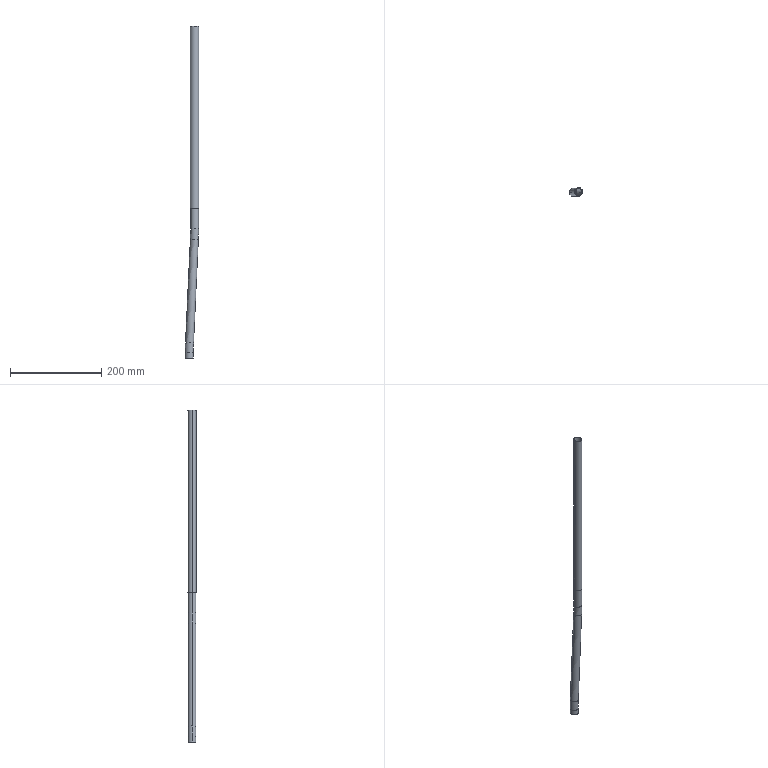Part | STEP file | Rear Chain Tube | 1 solid | 25 faces | box 29.277 x 18 x 727.809 mm | volume 34807 mm3 | cylinder 14 | torus 8 | plane 3 | commonest cylinder face diameters 16 x6 17.555 x6 18 x2
STEP:
#1=CARTESIAN_POINT('',(0.,0.,0.));
#2=DIRECTION('',(0.,0.,1.));
#3=DIRECTION('',(1.,0.,0.));
#4=AXIS2_PLACEMENT_3D('',#1,#2,#3);
#5=CARTESIAN_POINT('',(-8.,0.,-444.72));
#6=VERTEX_POINT('',#5);
#7=CARTESIAN_POINT('',(-8.527,0.,-467.477));
#8=VERTEX_POINT('',#7);
#9=CARTESIAN_POINT('',(-500.,0.,-444.72));
#10=DIRECTION('',(0.,1.,0.));
#11=DIRECTION('',(0.,0.,1.));
#12=AXIS2_PLACEMENT_3D('',#9,#10,#11);
#13=CIRCLE('',#12,492.);
#14=CARTESIAN_POINT('',(-500.,0.,-444.72));
#15=DIRECTION('',(0.,1.,0.));
#16=DIRECTION('',(0.,0.,1.));
#17=AXIS2_PLACEMENT_3D('',#14,#15,#16);
#18=TOROIDAL_SURFACE('',#17,500.,8.);
#19=CARTESIAN_POINT('',(0.,3.142));
#20=DIRECTION('',(1.,0.));
#21=VECTOR('',#20,1.);
#22=LINE('',#19,#21);
#23=(GEOMETRIC_REPRESENTATION_CONTEXT(2)PARAMETRIC_REPRESENTATION_CONTEXT()REPRESENTATION_CONTEXT('',''));
#24=DEFINITIONAL_REPRESENTATION('',(#22),#23);
#25=PCURVE('',#18,#24);
#26=CARTESIAN_POINT('',(-500.,0.,-444.72));
#27=DIRECTION('',(0.,1.,0.));
#28=DIRECTION('',(0.,0.,1.));
#29=AXIS2_PLACEMENT_3D('',#26,#27,#28);
#30=TOROIDAL_SURFACE('',#29,500.,8.);
#31=CARTESIAN_POINT('',(0.,3.142));
#32=DIRECTION('',(1.,0.));
#33=VECTOR('',#32,1.);
#34=LINE('',#31,#33);
#35=(GEOMETRIC_REPRESENTATION_CONTEXT(2)PARAMETRIC_REPRESENTATION_CONTEXT()REPRESENTATION_CONTEXT('',''));
#36=DEFINITIONAL_REPRESENTATION('',(#34),#35);
#37=PCURVE('',#30,#36);
#38=SURFACE_CURVE('',#13,(#25,#37),.PCURVE_S1.);
#39=EDGE_CURVE('',#6,#8,#38,.T.);
#40=ORIENTED_EDGE('',*,*,#39,.T.);
#41=CARTESIAN_POINT('',(7.456,0.,-468.217));
#42=VERTEX_POINT('',#41);
#43=CARTESIAN_POINT('',(-0.5351,0.,-467.847));
#44=DIRECTION('',(-0.04625,0.,-0.9989));
#45=DIRECTION('',(-0.9989,0.,0.04625));
#46=AXIS2_PLACEMENT_3D('',#43,#44,#45);
#47=CIRCLE('',#46,8.);
#48=CARTESIAN_POINT('',(1.617,9.425));
#49=DIRECTION('',(0.,-1.));
#50=VECTOR('',#49,1.);
#51=LINE('',#48,#50);
#52=(GEOMETRIC_REPRESENTATION_CONTEXT(2)PARAMETRIC_REPRESENTATION_CONTEXT()REPRESENTATION_CONTEXT('',''));
#53=DEFINITIONAL_REPRESENTATION('',(#51),#52);
#54=PCURVE('',#18,#53);
#55=CARTESIAN_POINT('',(-0.5351,0.,-467.847));
#56=DIRECTION('',(-0.04625,0.,-0.9989));
#57=DIRECTION('',(-0.9989,0.,0.04625));
#58=AXIS2_PLACEMENT_3D('',#55,#56,#57);
#59=CYLINDRICAL_SURFACE('',#58,8.);
#60=CARTESIAN_POINT('',(0.,0.));
#61=DIRECTION('',(1.,0.));
#62=VECTOR('',#61,1.);
#63=LINE('',#60,#62);
#64=(GEOMETRIC_REPRESENTATION_CONTEXT(2)PARAMETRIC_REPRESENTATION_CONTEXT()REPRESENTATION_CONTEXT('',''));
#65=DEFINITIONAL_REPRESENTATION('',(#63),#64);
#66=PCURVE('',#59,#65);
#67=SURFACE_CURVE('',#47,(#54,#66),.PCURVE_S1.);
#68=EDGE_CURVE('',#42,#8,#67,.T.);
#69=ORIENTED_EDGE('',*,*,#68,.F.);
#70=CARTESIAN_POINT('',(8.,0.,-444.72));
#71=VERTEX_POINT('',#70);
#72=CARTESIAN_POINT('',(-500.,0.,-444.72));
#73=DIRECTION('',(0.,1.,0.));
#74=DIRECTION('',(0.,0.,1.));
#75=AXIS2_PLACEMENT_3D('',#72,#73,#74);
#76=CIRCLE('',#75,508.);
#77=CARTESIAN_POINT('',(0.,6.283));
#78=DIRECTION('',(1.,0.));
#79=VECTOR('',#78,1.);
#80=LINE('',#77,#79);
#81=(GEOMETRIC_REPRESENTATION_CONTEXT(2)PARAMETRIC_REPRESENTATION_CONTEXT()REPRESENTATION_CONTEXT('',''));
#82=DEFINITIONAL_REPRESENTATION('',(#80),#81);
#83=PCURVE('',#18,#82);
#84=CARTESIAN_POINT('',(0.,0.));
#85=DIRECTION('',(1.,0.));
#86=VECTOR('',#85,1.);
#87=LINE('',#84,#86);
#88=(GEOMETRIC_REPRESENTATION_CONTEXT(2)PARAMETRIC_REPRESENTATION_CONTEXT()REPRESENTATION_CONTEXT('',''));
#89=DEFINITIONAL_REPRESENTATION('',(#87),#88);
#90=PCURVE('',#30,#89);
#91=SURFACE_CURVE('',#76,(#83,#90),.PCURVE_S1.);
#92=EDGE_CURVE('',#71,#42,#91,.T.);
#93=ORIENTED_EDGE('',*,*,#92,.F.);
#94=CARTESIAN_POINT('',(0.,0.,-444.72));
#95=DIRECTION('',(0.,0.,-1.));
#96=DIRECTION('',(-1.,0.,0.));
#97=AXIS2_PLACEMENT_3D('',#94,#95,#96);
#98=CIRCLE('',#97,8.);
#99=CARTESIAN_POINT('',(1.571,9.425));
#100=DIRECTION('',(0.,-1.));
#101=VECTOR('',#100,1.);
#102=LINE('',#99,#101);
#103=(GEOMETRIC_REPRESENTATION_CONTEXT(2)PARAMETRIC_REPRESENTATION_CONTEXT()REPRESENTATION_CONTEXT('',''));
#104=DEFINITIONAL_REPRESENTATION('',(#102),#103);
#105=PCURVE('',#18,#104);
#106=CARTESIAN_POINT('',(0.,0.,-400.));
#107=DIRECTION('',(0.,0.,1.));
#108=DIRECTION('',(1.,0.,0.));
#109=AXIS2_PLACEMENT_3D('',#106,#107,#108);
#110=CYLINDRICAL_SURFACE('',#109,8.);
#111=CARTESIAN_POINT('',(9.425,-44.72));
#112=DIRECTION('',(-1.,0.));
#113=VECTOR('',#112,1.);
#114=LINE('',#111,#113);
#115=(GEOMETRIC_REPRESENTATION_CONTEXT(2)PARAMETRIC_REPRESENTATION_CONTEXT()REPRESENTATION_CONTEXT('',''));
#116=DEFINITIONAL_REPRESENTATION('',(#114),#115);
#117=PCURVE('',#110,#116);
#118=SURFACE_CURVE('',#98,(#105,#117),.PCURVE_S1.);
#119=EDGE_CURVE('',#71,#6,#118,.T.);
#120=ORIENTED_EDGE('',*,*,#119,.T.);
#121=EDGE_LOOP('',(#40,#69,#93,#120));
#122=FACE_BOUND('',#121,.F.);
#123=ADVANCED_FACE('',(#122),#18,.F.);
#124=CARTESIAN_POINT('',(-8.777,0.,-444.72));
#125=VERTEX_POINT('',#124);
#126=CARTESIAN_POINT('',(8.777,0.,-444.72));
#127=VERTEX_POINT('',#126);
#128=CARTESIAN_POINT('',(0.,0.,-444.72));
#129=DIRECTION('',(0.,0.,-1.));
#130=DIRECTION('',(-1.,0.,0.));
#131=AXIS2_PLACEMENT_3D('',#128,#129,#130);
#132=CIRCLE('',#131,8.777);
#133=CARTESIAN_POINT('',(-500.,0.,-444.72));
#134=DIRECTION('',(0.,1.,0.));
#135=DIRECTION('',(0.,0.,1.));
#136=AXIS2_PLACEMENT_3D('',#133,#134,#135);
#137=TOROIDAL_SURFACE('',#136,500.,8.777);
#138=CARTESIAN_POINT('',(1.571,3.142));
#139=DIRECTION('',(0.,-1.));
#140=VECTOR('',#139,1.);
#141=LINE('',#138,#140);
#142=(GEOMETRIC_REPRESENTATION_CONTEXT(2)PARAMETRIC_REPRESENTATION_CONTEXT()REPRESENTATION_CONTEXT('',''));
#143=DEFINITIONAL_REPRESENTATION('',(#141),#142);
#144=PCURVE('',#137,#143);
#145=CARTESIAN_POINT('',(0.,0.,-444.72));
#146=DIRECTION('',(0.,0.,1.));
#147=DIRECTION('',(1.,0.,0.));
#148=AXIS2_PLACEMENT_3D('',#145,#146,#147);
#149=CYLINDRICAL_SURFACE('',#148,8.777);
#150=CARTESIAN_POINT('',(3.142,0.));
#151=DIRECTION('',(-1.,0.));
#152=VECTOR('',#151,1.);
#153=LINE('',#150,#152);
#154=(GEOMETRIC_REPRESENTATION_CONTEXT(2)PARAMETRIC_REPRESENTATION_CONTEXT()REPRESENTATION_CONTEXT('',''));
#155=DEFINITIONAL_REPRESENTATION('',(#153),#154);
#156=PCURVE('',#149,#155);
#157=SURFACE_CURVE('',#132,(#144,#156),.PCURVE_S1.);
#158=EDGE_CURVE('',#125,#127,#157,.T.);
#159=ORIENTED_EDGE('',*,*,#158,.T.);
#160=CARTESIAN_POINT('',(8.233,0.,-468.253));
#161=VERTEX_POINT('',#160);
#162=CARTESIAN_POINT('',(-500.,0.,-444.72));
#163=DIRECTION('',(0.,1.,0.));
#164=DIRECTION('',(0.,0.,1.));
#165=AXIS2_PLACEMENT_3D('',#162,#163,#164);
#166=CIRCLE('',#165,508.777);
#167=CARTESIAN_POINT('',(0.,0.));
#168=DIRECTION('',(1.,0.));
#169=VECTOR('',#168,1.);
#170=LINE('',#167,#169);
#171=(GEOMETRIC_REPRESENTATION_CONTEXT(2)PARAMETRIC_REPRESENTATION_CONTEXT()REPRESENTATION_CONTEXT('',''));
#172=DEFINITIONAL_REPRESENTATION('',(#170),#171);
#173=PCURVE('',#137,#172);
#174=CARTESIAN_POINT('',(-500.,0.,-444.72));
#175=DIRECTION('',(0.,1.,0.));
#176=DIRECTION('',(0.,0.,1.));
#177=AXIS2_PLACEMENT_3D('',#174,#175,#176);
#178=TOROIDAL_SURFACE('',#177,500.,8.777);
#179=CARTESIAN_POINT('',(0.,6.283));
#180=DIRECTION('',(1.,0.));
#181=VECTOR('',#180,1.);
#182=LINE('',#179,#181);
#183=(GEOMETRIC_REPRESENTATION_CONTEXT(2)PARAMETRIC_REPRESENTATION_CONTEXT()REPRESENTATION_CONTEXT('',''));
#184=DEFINITIONAL_REPRESENTATION('',(#182),#183);
#185=PCURVE('',#178,#184);
#186=SURFACE_CURVE('',#166,(#173,#185),.PCURVE_S1.);
#187=EDGE_CURVE('',#127,#161,#186,.T.);
#188=ORIENTED_EDGE('',*,*,#187,.T.);
#189=CARTESIAN_POINT('',(-9.303,0.,-467.441));
#190=VERTEX_POINT('',#189);
#191=CARTESIAN_POINT('',(-0.5351,0.,-467.847));
#192=DIRECTION('',(-0.04625,0.,-0.9989));
#193=DIRECTION('',(-0.9989,0.,0.04625));
#194=AXIS2_PLACEMENT_3D('',#191,#192,#193);
#195=CIRCLE('',#194,8.777);
#196=CARTESIAN_POINT('',(1.617,3.142));
#197=DIRECTION('',(0.,-1.));
#198=VECTOR('',#197,1.);
#199=LINE('',#196,#198);
#200=(GEOMETRIC_REPRESENTATION_CONTEXT(2)PARAMETRIC_REPRESENTATION_CONTEXT()REPRESENTATION_CONTEXT('',''));
#201=DEFINITIONAL_REPRESENTATION('',(#199),#200);
#202=PCURVE('',#137,#201);
#203=CARTESIAN_POINT('',(-0.5351,0.,-467.847));
#204=DIRECTION('',(-0.04625,0.,-0.9989));
#205=DIRECTION('',(-0.9989,0.,0.04625));
#206=AXIS2_PLACEMENT_3D('',#203,#204,#205);
#207=CYLINDRICAL_SURFACE('',#206,8.777);
#208=CARTESIAN_POINT('',(0.,0.));
#209=DIRECTION('',(1.,0.));
#210=VECTOR('',#209,1.);
#211=LINE('',#208,#210);
#212=(GEOMETRIC_REPRESENTATION_CONTEXT(2)PARAMETRIC_REPRESENTATION_CONTEXT()REPRESENTATION_CONTEXT('',''));
#213=DEFINITIONAL_REPRESENTATION('',(#211),#212);
#214=PCURVE('',#207,#213);
#215=SURFACE_CURVE('',#195,(#202,#214),.PCURVE_S1.);
#216=EDGE_CURVE('',#190,#161,#215,.T.);
#217=ORIENTED_EDGE('',*,*,#216,.F.);
#218=CARTESIAN_POINT('',(-500.,0.,-444.72));
#219=DIRECTION('',(0.,1.,0.));
#220=DIRECTION('',(0.,0.,1.));
#221=AXIS2_PLACEMENT_3D('',#218,#219,#220);
#222=CIRCLE('',#221,491.223);
#223=CARTESIAN_POINT('',(0.,3.142));
#224=DIRECTION('',(1.,0.));
#225=VECTOR('',#224,1.);
#226=LINE('',#223,#225);
#227=(GEOMETRIC_REPRESENTATION_CONTEXT(2)PARAMETRIC_REPRESENTATION_CONTEXT()REPRESENTATION_CONTEXT('',''));
#228=DEFINITIONAL_REPRESENTATION('',(#226),#227);
#229=PCURVE('',#137,#228);
#230=CARTESIAN_POINT('',(0.,3.142));
#231=DIRECTION('',(1.,0.));
#232=VECTOR('',#231,1.);
#233=LINE('',#230,#232);
#234=(GEOMETRIC_REPRESENTATION_CONTEXT(2)PARAMETRIC_REPRESENTATION_CONTEXT()REPRESENTATION_CONTEXT('',''));
#235=DEFINITIONAL_REPRESENTATION('',(#233),#234);
#236=PCURVE('',#178,#235);
#237=SURFACE_CURVE('',#222,(#229,#236),.PCURVE_S1.);
#238=EDGE_CURVE('',#125,#190,#237,.T.);
#239=ORIENTED_EDGE('',*,*,#238,.F.);
#240=EDGE_LOOP('',(#159,#188,#217,#239));
#241=FACE_BOUND('',#240,.T.);
#242=ADVANCED_FACE('',(#241),#137,.T.);
#243=CARTESIAN_POINT('',(-2.973,0.,-693.469));
#244=VERTEX_POINT('',#243);
#245=CARTESIAN_POINT('',(-3.5,0.,-716.225));
#246=VERTEX_POINT('',#245);
#247=CARTESIAN_POINT('',(488.5,0.,-716.225));
#248=DIRECTION('',(0.,-1.,0.));
#249=DIRECTION('',(0.,0.,-1.));
#250=AXIS2_PLACEMENT_3D('',#247,#248,#249);
#251=CIRCLE('',#250,492.);
#252=CARTESIAN_POINT('',(488.5,0.,-716.225));
#253=DIRECTION('',(0.,-1.,0.));
#254=DIRECTION('',(0.,0.,-1.));
#255=AXIS2_PLACEMENT_3D('',#252,#253,#254);
#256=TOROIDAL_SURFACE('',#255,500.,8.);
#257=CARTESIAN_POINT('',(0.,3.142));
#258=DIRECTION('',(1.,0.));
#259=VECTOR('',#258,1.);
#260=LINE('',#257,#259);
#261=(GEOMETRIC_REPRESENTATION_CONTEXT(2)PARAMETRIC_REPRESENTATION_CONTEXT()REPRESENTATION_CONTEXT('',''));
#262=DEFINITIONAL_REPRESENTATION('',(#260),#261);
#263=PCURVE('',#256,#262);
#264=CARTESIAN_POINT('',(488.5,0.,-716.225));
#265=DIRECTION('',(0.,-1.,0.));
#266=DIRECTION('',(0.,0.,-1.));
#267=AXIS2_PLACEMENT_3D('',#264,#265,#266);
#268=TOROIDAL_SURFACE('',#267,500.,8.);
#269=CARTESIAN_POINT('',(0.,3.142));
#270=DIRECTION('',(1.,0.));
#271=VECTOR('',#270,1.);
#272=LINE('',#269,#271);
#273=(GEOMETRIC_REPRESENTATION_CONTEXT(2)PARAMETRIC_REPRESENTATION_CONTEXT()REPRESENTATION_CONTEXT('',''));
#274=DEFINITIONAL_REPRESENTATION('',(#272),#273);
#275=PCURVE('',#268,#274);
#276=SURFACE_CURVE('',#251,(#263,#275),.PCURVE_S1.);
#277=EDGE_CURVE('',#244,#246,#276,.T.);
#278=ORIENTED_EDGE('',*,*,#277,.T.);
#279=CARTESIAN_POINT('',(-19.5,0.,-716.225));
#280=VERTEX_POINT('',#279);
#281=CARTESIAN_POINT('',(-11.5,0.,-716.225));
#282=DIRECTION('',(0.,0.,-1.));
#283=DIRECTION('',(-1.,0.,0.));
#284=AXIS2_PLACEMENT_3D('',#281,#282,#283);
#285=CIRCLE('',#284,8.);
#286=CARTESIAN_POINT('',(4.712,6.283));
#287=DIRECTION('',(0.,-1.));
#288=VECTOR('',#287,1.);
#289=LINE('',#286,#288);
#290=(GEOMETRIC_REPRESENTATION_CONTEXT(2)PARAMETRIC_REPRESENTATION_CONTEXT()REPRESENTATION_CONTEXT('',''));
#291=DEFINITIONAL_REPRESENTATION('',(#289),#290);
#292=PCURVE('',#256,#291);
#293=CARTESIAN_POINT('',(-11.5,0.,-716.225));
#294=DIRECTION('',(0.,0.,-1.));
#295=DIRECTION('',(-1.,0.,0.));
#296=AXIS2_PLACEMENT_3D('',#293,#294,#295);
#297=CYLINDRICAL_SURFACE('',#296,8.);
#298=CARTESIAN_POINT('',(0.,0.));
#299=DIRECTION('',(1.,0.));
#300=VECTOR('',#299,1.);
#301=LINE('',#298,#300);
#302=(GEOMETRIC_REPRESENTATION_CONTEXT(2)PARAMETRIC_REPRESENTATION_CONTEXT()REPRESENTATION_CONTEXT('',''));
#303=DEFINITIONAL_REPRESENTATION('',(#301),#302);
#304=PCURVE('',#297,#303);
#305=SURFACE_CURVE('',#285,(#292,#304),.PCURVE_S1.);
#306=EDGE_CURVE('',#280,#246,#305,.T.);
#307=ORIENTED_EDGE('',*,*,#306,.F.);
#308=CARTESIAN_POINT('',(-18.956,0.,-692.729));
#309=VERTEX_POINT('',#308);
#310=CARTESIAN_POINT('',(488.5,0.,-716.225));
#311=DIRECTION('',(0.,-1.,0.));
#312=DIRECTION('',(0.,0.,-1.));
#313=AXIS2_PLACEMENT_3D('',#310,#311,#312);
#314=CIRCLE('',#313,508.);
#315=CARTESIAN_POINT('',(0.,6.283));
#316=DIRECTION('',(1.,0.));
#317=VECTOR('',#316,1.);
#318=LINE('',#315,#317);
#319=(GEOMETRIC_REPRESENTATION_CONTEXT(2)PARAMETRIC_REPRESENTATION_CONTEXT()REPRESENTATION_CONTEXT('',''));
#320=DEFINITIONAL_REPRESENTATION('',(#318),#319);
#321=PCURVE('',#256,#320);
#322=CARTESIAN_POINT('',(0.,0.));
#323=DIRECTION('',(1.,0.));
#324=VECTOR('',#323,1.);
#325=LINE('',#322,#324);
#326=(GEOMETRIC_REPRESENTATION_CONTEXT(2)PARAMETRIC_REPRESENTATION_CONTEXT()REPRESENTATION_CONTEXT('',''));
#327=DEFINITIONAL_REPRESENTATION('',(#325),#326);
#328=PCURVE('',#268,#327);
#329=SURFACE_CURVE('',#314,(#321,#328),.PCURVE_S1.);
#330=EDGE_CURVE('',#309,#280,#329,.T.);
#331=ORIENTED_EDGE('',*,*,#330,.F.);
#332=CARTESIAN_POINT('',(-10.965,0.,-693.099));
#333=DIRECTION('',(-0.04625,0.,-0.9989));
#334=DIRECTION('',(-0.9989,0.,0.04625));
#335=AXIS2_PLACEMENT_3D('',#332,#333,#334);
#336=CIRCLE('',#335,8.);
#337=CARTESIAN_POINT('',(4.666,6.283));
#338=DIRECTION('',(0.,-1.));
#339=VECTOR('',#338,1.);
#340=LINE('',#337,#339);
#341=(GEOMETRIC_REPRESENTATION_CONTEXT(2)PARAMETRIC_REPRESENTATION_CONTEXT()REPRESENTATION_CONTEXT('',''));
#342=DEFINITIONAL_REPRESENTATION('',(#340),#341);
#343=PCURVE('',#256,#342);
#344=CARTESIAN_POINT('',(-0.5351,0.,-467.847));
#345=DIRECTION('',(-0.04625,0.,-0.9989));
#346=DIRECTION('',(-0.9989,0.,0.04625));
#347=AXIS2_PLACEMENT_3D('',#344,#345,#346);
#348=CYLINDRICAL_SURFACE('',#347,8.);
#349=CARTESIAN_POINT('',(0.,225.493));
#350=DIRECTION('',(1.,0.));
#351=VECTOR('',#350,1.);
#352=LINE('',#349,#351);
#353=(GEOMETRIC_REPRESENTATION_CONTEXT(2)PARAMETRIC_REPRESENTATION_CONTEXT()REPRESENTATION_CONTEXT('',''));
#354=DEFINITIONAL_REPRESENTATION('',(#352),#353);
#355=PCURVE('',#348,#354);
#356=SURFACE_CURVE('',#336,(#343,#355),.PCURVE_S1.);
#357=EDGE_CURVE('',#309,#244,#356,.T.);
#358=ORIENTED_EDGE('',*,*,#357,.T.);
#359=EDGE_LOOP('',(#278,#307,#331,#358));
#360=FACE_BOUND('',#359,.F.);
#361=ADVANCED_FACE('',(#360),#256,.F.);
#362=CARTESIAN_POINT('',(-2.197,0.,-693.505));
#363=VERTEX_POINT('',#362);
#364=CARTESIAN_POINT('',(-19.733,0.,-692.693));
#365=VERTEX_POINT('',#364);
#366=CARTESIAN_POINT('',(-10.965,0.,-693.099));
#367=DIRECTION('',(-0.04625,0.,-0.9989));
#368=DIRECTION('',(-0.9989,0.,0.04625));
#369=AXIS2_PLACEMENT_3D('',#366,#367,#368);
#370=CIRCLE('',#369,8.777);
#371=CARTESIAN_POINT('',(488.5,0.,-716.225));
#372=DIRECTION('',(0.,-1.,0.));
#373=DIRECTION('',(0.,0.,-1.));
#374=AXIS2_PLACEMENT_3D('',#371,#372,#373);
#375=TOROIDAL_SURFACE('',#374,500.,8.777);
#376=CARTESIAN_POINT('',(4.666,6.283));
#377=DIRECTION('',(0.,-1.));
#378=VECTOR('',#377,1.);
#379=LINE('',#376,#378);
#380=(GEOMETRIC_REPRESENTATION_CONTEXT(2)PARAMETRIC_REPRESENTATION_CONTEXT()REPRESENTATION_CONTEXT('',''));
#381=DEFINITIONAL_REPRESENTATION('',(#379),#380);
#382=PCURVE('',#375,#381);
#383=CARTESIAN_POINT('',(-0.5351,0.,-467.847));
#384=DIRECTION('',(-0.04625,0.,-0.9989));
#385=DIRECTION('',(-0.9989,0.,0.04625));
#386=AXIS2_PLACEMENT_3D('',#383,#384,#385);
#387=CYLINDRICAL_SURFACE('',#386,8.777);
#388=CARTESIAN_POINT('',(0.,225.493));
#389=DIRECTION('',(1.,0.));
#390=VECTOR('',#389,1.);
#391=LINE('',#388,#390);
#392=(GEOMETRIC_REPRESENTATION_CONTEXT(2)PARAMETRIC_REPRESENTATION_CONTEXT()REPRESENTATION_CONTEXT('',''));
#393=DEFINITIONAL_REPRESENTATION('',(#391),#392);
#394=PCURVE('',#387,#393);
#395=SURFACE_CURVE('',#370,(#382,#394),.PCURVE_S1.);
#396=EDGE_CURVE('',#363,#365,#395,.T.);
#397=ORIENTED_EDGE('',*,*,#396,.T.);
#398=CARTESIAN_POINT('',(-20.277,0.,-716.225));
#399=VERTEX_POINT('',#398);
#400=CARTESIAN_POINT('',(488.5,0.,-716.225));
#401=DIRECTION('',(0.,-1.,0.));
#402=DIRECTION('',(0.,0.,-1.));
#403=AXIS2_PLACEMENT_3D('',#400,#401,#402);
#404=CIRCLE('',#403,508.777);
#405=CARTESIAN_POINT('',(0.,0.));
#406=DIRECTION('',(1.,0.));
#407=VECTOR('',#406,1.);
#408=LINE('',#405,#407);
#409=(GEOMETRIC_REPRESENTATION_CONTEXT(2)PARAMETRIC_REPRESENTATION_CONTEXT()REPRESENTATION_CONTEXT('',''));
#410=DEFINITIONAL_REPRESENTATION('',(#408),#409);
#411=PCURVE('',#375,#410);
#412=CARTESIAN_POINT('',(488.5,0.,-716.225));
#413=DIRECTION('',(0.,-1.,0.));
#414=DIRECTION('',(0.,0.,-1.));
#415=AXIS2_PLACEMENT_3D('',#412,#413,#414);
#416=TOROIDAL_SURFACE('',#415,500.,8.777);
#417=CARTESIAN_POINT('',(0.,6.283));
#418=DIRECTION('',(1.,0.));
#419=VECTOR('',#418,1.);
#420=LINE('',#417,#419);
#421=(GEOMETRIC_REPRESENTATION_CONTEXT(2)PARAMETRIC_REPRESENTATION_CONTEXT()REPRESENTATION_CONTEXT('',''));
#422=DEFINITIONAL_REPRESENTATION('',(#420),#421);
#423=PCURVE('',#416,#422);
#424=SURFACE_CURVE('',#404,(#411,#423),.PCURVE_S1.);
#425=EDGE_CURVE('',#365,#399,#424,.T.);
#426=ORIENTED_EDGE('',*,*,#425,.T.);
#427=CARTESIAN_POINT('',(-2.723,0.,-716.225));
#428=VERTEX_POINT('',#427);
#429=CARTESIAN_POINT('',(-11.5,0.,-716.225));
#430=DIRECTION('',(0.,0.,-1.));
#431=DIRECTION('',(-1.,0.,0.));
#432=AXIS2_PLACEMENT_3D('',#429,#430,#431);
#433=CIRCLE('',#432,8.777);
#434=CARTESIAN_POINT('',(4.712,6.283));
#435=DIRECTION('',(0.,-1.));
#436=VECTOR('',#435,1.);
#437=LINE('',#434,#436);
#438=(GEOMETRIC_REPRESENTATION_CONTEXT(2)PARAMETRIC_REPRESENTATION_CONTEXT()REPRESENTATION_CONTEXT('',''));
#439=DEFINITIONAL_REPRESENTATION('',(#437),#438);
#440=PCURVE('',#375,#439);
#441=CARTESIAN_POINT('',(-11.5,0.,-716.225));
#442=DIRECTION('',(0.,0.,-1.));
#443=DIRECTION('',(-1.,0.,0.));
#444=AXIS2_PLACEMENT_3D('',#441,#442,#443);
#445=CYLINDRICAL_SURFACE('',#444,8.777);
#446=CARTESIAN_POINT('',(0.,0.));
#447=DIRECTION('',(1.,0.));
#448=VECTOR('',#447,1.);
#449=LINE('',#446,#448);
#450=(GEOMETRIC_REPRESENTATION_CONTEXT(2)PARAMETRIC_REPRESENTATION_CONTEXT()REPRESENTATION_CONTEXT('',''));
#451=DEFINITIONAL_REPRESENTATION('',(#449),#450);
#452=PCURVE('',#445,#451);
#453=SURFACE_CURVE('',#433,(#440,#452),.PCURVE_S1.);
#454=EDGE_CURVE('',#428,#399,#453,.T.);
#455=ORIENTED_EDGE('',*,*,#454,.F.);
#456=CARTESIAN_POINT('',(488.5,0.,-716.225));
#457=DIRECTION('',(0.,-1.,0.));
#458=DIRECTION('',(0.,0.,-1.));
#459=AXIS2_PLACEMENT_3D('',#456,#457,#458);
#460=CIRCLE('',#459,491.223);
#461=CARTESIAN_POINT('',(0.,3.142));
#462=DIRECTION('',(1.,0.));
#463=VECTOR('',#462,1.);
#464=LINE('',#461,#463);
#465=(GEOMETRIC_REPRESENTATION_CONTEXT(2)PARAMETRIC_REPRESENTATION_CONTEXT()REPRESENTATION_CONTEXT('',''));
#466=DEFINITIONAL_REPRESENTATION('',(#464),#465);
#467=PCURVE('',#375,#466);
#468=CARTESIAN_POINT('',(0.,3.142));
#469=DIRECTION('',(1.,0.));
#470=VECTOR('',#469,1.);
#471=LINE('',#468,#470);
#472=(GEOMETRIC_REPRESENTATION_CONTEXT(2)PARAMETRIC_REPRESENTATION_CONTEXT()REPRESENTATION_CONTEXT('',''));
#473=DEFINITIONAL_REPRESENTATION('',(#471),#472);
#474=PCURVE('',#416,#473);
#475=SURFACE_CURVE('',#460,(#467,#474),.PCURVE_S1.);
#476=EDGE_CURVE('',#363,#428,#475,.T.);
#477=ORIENTED_EDGE('',*,*,#476,.F.);
#478=EDGE_LOOP('',(#397,#426,#455,#477));
#479=FACE_BOUND('',#478,.T.);
#480=ADVANCED_FACE('',(#479),#375,.T.);
#481=ORIENTED_EDGE('',*,*,#158,.F.);
#482=CARTESIAN_POINT('',(-8.777,0.,-400.));
#483=VERTEX_POINT('',#482);
#484=CARTESIAN_POINT('',(-8.777,0.,-444.72));
#485=DIRECTION('',(0.,0.,1.));
#486=VECTOR('',#485,1.);
#487=LINE('',#484,#486);
#488=CARTESIAN_POINT('',(3.142,0.));
#489=DIRECTION('',(0.,1.));
#490=VECTOR('',#489,1.);
#491=LINE('',#488,#490);
#492=(GEOMETRIC_REPRESENTATION_CONTEXT(2)PARAMETRIC_REPRESENTATION_CONTEXT()REPRESENTATION_CONTEXT('',''));
#493=DEFINITIONAL_REPRESENTATION('',(#491),#492);
#494=PCURVE('',#149,#493);
#495=CARTESIAN_POINT('',(0.,0.,-444.72));
#496=DIRECTION('',(0.,0.,1.));
#497=DIRECTION('',(1.,0.,0.));
#498=AXIS2_PLACEMENT_3D('',#495,#496,#497);
#499=CYLINDRICAL_SURFACE('',#498,8.777);
#500=CARTESIAN_POINT('',(3.142,0.));
#501=DIRECTION('',(0.,1.));
#502=VECTOR('',#501,1.);
#503=LINE('',#500,#502);
#504=(GEOMETRIC_REPRESENTATION_CONTEXT(2)PARAMETRIC_REPRESENTATION_CONTEXT()REPRESENTATION_CONTEXT('',''));
#505=DEFINITIONAL_REPRESENTATION('',(#503),#504);
#506=PCURVE('',#499,#505);
#507=SURFACE_CURVE('',#487,(#494,#506),.PCURVE_S1.);
#508=EDGE_CURVE('',#125,#483,#507,.T.);
#509=ORIENTED_EDGE('',*,*,#508,.T.);
#510=CARTESIAN_POINT('',(8.777,0.,-400.));
#511=VERTEX_POINT('',#510);
#512=CARTESIAN_POINT('',(0.,0.,-400.));
#513=DIRECTION('',(0.,0.,-1.));
#514=DIRECTION('',(-1.,0.,0.));
#515=AXIS2_PLACEMENT_3D('',#512,#513,#514);
#516=CIRCLE('',#515,8.777);
#517=CARTESIAN_POINT('',(3.142,44.72));
#518=DIRECTION('',(-1.,0.));
#519=VECTOR('',#518,1.);
#520=LINE('',#517,#519);
#521=(GEOMETRIC_REPRESENTATION_CONTEXT(2)PARAMETRIC_REPRESENTATION_CONTEXT()REPRESENTATION_CONTEXT('',''));
#522=DEFINITIONAL_REPRESENTATION('',(#520),#521);
#523=PCURVE('',#149,#522);
#524=CARTESIAN_POINT('',(0.,0.,-400.));
#525=DIRECTION('',(0.,0.,1.));
#526=DIRECTION('',(1.,0.,0.));
#527=AXIS2_PLACEMENT_3D('',#524,#525,#526);
#528=PLANE('',#527);
#529=CARTESIAN_POINT('',(-8.777,0.));
#530=CARTESIAN_POINT('',(-8.777,15.203));
#531=CARTESIAN_POINT('',(4.389,7.602));
#532=CARTESIAN_POINT('',(17.555,0.));
#533=CARTESIAN_POINT('',(4.389,-7.602));
#534=CARTESIAN_POINT('',(-8.777,-15.203));
#535=CARTESIAN_POINT('',(-8.777,0.));
#536=(BOUNDED_CURVE()B_SPLINE_CURVE(2,(#529,#530,#531,#532,#533,#534,#535),.UNSPECIFIED.,.T.,.F.)B_SPLINE_CURVE_WITH_KNOTS((1,2,2,2,2,1),(-2.094,0.,2.094,4.189,6.283,8.378),.UNSPECIFIED.)CURVE()GEOMETRIC_REPRESENTATION_ITEM()RATIONAL_B_SPLINE_CURVE((1.,0.5,1.,0.5,1.,0.5,1.))REPRESENTATION_ITEM(''));
#537=(GEOMETRIC_REPRESENTATION_CONTEXT(2)PARAMETRIC_REPRESENTATION_CONTEXT()REPRESENTATION_CONTEXT('',''));
#538=DEFINITIONAL_REPRESENTATION('',(#536),#537);
#539=PCURVE('',#528,#538);
#540=SURFACE_CURVE('',#516,(#523,#539),.PCURVE_S1.);
#541=EDGE_CURVE('',#483,#511,#540,.T.);
#542=ORIENTED_EDGE('',*,*,#541,.T.);
#543=CARTESIAN_POINT('',(8.777,0.,-444.72));
#544=DIRECTION('',(0.,0.,1.));
#545=VECTOR('',#544,1.);
#546=LINE('',#543,#545);
#547=CARTESIAN_POINT('',(0.,0.));
#548=DIRECTION('',(0.,1.));
#549=VECTOR('',#548,1.);
#550=LINE('',#547,#549);
#551=(GEOMETRIC_REPRESENTATION_CONTEXT(2)PARAMETRIC_REPRESENTATION_CONTEXT()REPRESENTATION_CONTEXT('',''));
#552=DEFINITIONAL_REPRESENTATION('',(#550),#551);
#553=PCURVE('',#149,#552);
#554=CARTESIAN_POINT('',(6.283,0.));
#555=DIRECTION('',(0.,1.));
#556=VECTOR('',#555,1.);
#557=LINE('',#554,#556);
#558=(GEOMETRIC_REPRESENTATION_CONTEXT(2)PARAMETRIC_REPRESENTATION_CONTEXT()REPRESENTATION_CONTEXT('',''));
#559=DEFINITIONAL_REPRESENTATION('',(#557),#558);
#560=PCURVE('',#499,#559);
#561=SURFACE_CURVE('',#546,(#553,#560),.PCURVE_S1.);
#562=EDGE_CURVE('',#127,#511,#561,.T.);
#563=ORIENTED_EDGE('',*,*,#562,.F.);
#564=EDGE_LOOP('',(#481,#509,#542,#563));
#565=FACE_BOUND('',#564,.T.);
#566=ADVANCED_FACE('',(#565),#149,.T.);
#567=CARTESIAN_POINT('',(-8.527,0.,-467.477));
#568=DIRECTION('',(-0.04625,0.,-0.9989));
#569=VECTOR('',#568,1.);
#570=LINE('',#567,#569);
#571=CARTESIAN_POINT('',(6.283,0.));
#572=DIRECTION('',(0.,1.));
#573=VECTOR('',#572,1.);
#574=LINE('',#571,#573);
#575=(GEOMETRIC_REPRESENTATION_CONTEXT(2)PARAMETRIC_REPRESENTATION_CONTEXT()REPRESENTATION_CONTEXT('',''));
#576=DEFINITIONAL_REPRESENTATION('',(#574),#575);
#577=PCURVE('',#59,#576);
#578=CARTESIAN_POINT('',(0.,0.));
#579=DIRECTION('',(0.,1.));
#580=VECTOR('',#579,1.);
#581=LINE('',#578,#580);
#582=(GEOMETRIC_REPRESENTATION_CONTEXT(2)PARAMETRIC_REPRESENTATION_CONTEXT()REPRESENTATION_CONTEXT('',''));
#583=DEFINITIONAL_REPRESENTATION('',(#581),#582);
#584=PCURVE('',#348,#583);
#585=SURFACE_CURVE('',#570,(#577,#584),.PCURVE_S1.);
#586=EDGE_CURVE('',#8,#309,#585,.T.);
#587=ORIENTED_EDGE('',*,*,#586,.T.);
#588=CARTESIAN_POINT('',(-10.965,0.,-693.099));
#589=DIRECTION('',(-0.04625,0.,-0.9989));
#590=DIRECTION('',(-0.9989,0.,0.04625));
#591=AXIS2_PLACEMENT_3D('',#588,#589,#590);
#592=CIRCLE('',#591,8.);
#593=CARTESIAN_POINT('',(0.,225.493));
#594=DIRECTION('',(1.,0.));
#595=VECTOR('',#594,1.);
#596=LINE('',#593,#595);
#597=(GEOMETRIC_REPRESENTATION_CONTEXT(2)PARAMETRIC_REPRESENTATION_CONTEXT()REPRESENTATION_CONTEXT('',''));
#598=DEFINITIONAL_REPRESENTATION('',(#596),#597);
#599=PCURVE('',#59,#598);
#600=CARTESIAN_POINT('',(4.666,6.283));
#601=DIRECTION('',(0.,-1.));
#602=VECTOR('',#601,1.);
#603=LINE('',#600,#602);
#604=(GEOMETRIC_REPRESENTATION_CONTEXT(2)PARAMETRIC_REPRESENTATION_CONTEXT()REPRESENTATION_CONTEXT('',''));
#605=DEFINITIONAL_REPRESENTATION('',(#603),#604);
#606=PCURVE('',#268,#605);
#607=SURFACE_CURVE('',#592,(#599,#606),.PCURVE_S1.);
#608=EDGE_CURVE('',#244,#309,#607,.T.);
#609=ORIENTED_EDGE('',*,*,#608,.F.);
#610=CARTESIAN_POINT('',(7.456,0.,-468.217));
#611=DIRECTION('',(-0.04625,0.,-0.9989));
#612=VECTOR('',#611,1.);
#613=LINE('',#610,#612);
#614=CARTESIAN_POINT('',(3.142,0.));
#615=DIRECTION('',(0.,1.));
#616=VECTOR('',#615,1.);
#617=LINE('',#614,#616);
#618=(GEOMETRIC_REPRESENTATION_CONTEXT(2)PARAMETRIC_REPRESENTATION_CONTEXT()REPRESENTATION_CONTEXT('',''));
#619=DEFINITIONAL_REPRESENTATION('',(#617),#618);
#620=PCURVE('',#59,#619);
#621=CARTESIAN_POINT('',(3.142,0.));
#622=DIRECTION('',(0.,1.));
#623=VECTOR('',#622,1.);
#624=LINE('',#621,#623);
#625=(GEOMETRIC_REPRESENTATION_CONTEXT(2)PARAMETRIC_REPRESENTATION_CONTEXT()REPRESENTATION_CONTEXT('',''));
#626=DEFINITIONAL_REPRESENTATION('',(#624),#625);
#627=PCURVE('',#348,#626);
#628=SURFACE_CURVE('',#613,(#620,#627),.PCURVE_S1.);
#629=EDGE_CURVE('',#42,#244,#628,.T.);
#630=ORIENTED_EDGE('',*,*,#629,.F.);
#631=ORIENTED_EDGE('',*,*,#68,.T.);
#632=EDGE_LOOP('',(#587,#609,#630,#631));
#633=FACE_BOUND('',#632,.F.);
#634=ADVANCED_FACE('',(#633),#59,.F.);
#635=ORIENTED_EDGE('',*,*,#216,.T.);
#636=CARTESIAN_POINT('',(8.233,0.,-468.253));
#637=DIRECTION('',(-0.04625,0.,-0.9989));
#638=VECTOR('',#637,1.);
#639=LINE('',#636,#638);
#640=CARTESIAN_POINT('',(3.142,0.));
#641=DIRECTION('',(0.,1.));
#642=VECTOR('',#641,1.);
#643=LINE('',#640,#642);
#644=(GEOMETRIC_REPRESENTATION_CONTEXT(2)PARAMETRIC_REPRESENTATION_CONTEXT()REPRESENTATION_CONTEXT('',''));
#645=DEFINITIONAL_REPRESENTATION('',(#643),#644);
#646=PCURVE('',#207,#645);
#647=CARTESIAN_POINT('',(3.142,0.));
#648=DIRECTION('',(0.,1.));
#649=VECTOR('',#648,1.);
#650=LINE('',#647,#649);
#651=(GEOMETRIC_REPRESENTATION_CONTEXT(2)PARAMETRIC_REPRESENTATION_CONTEXT()REPRESENTATION_CONTEXT('',''));
#652=DEFINITIONAL_REPRESENTATION('',(#650),#651);
#653=PCURVE('',#387,#652);
#654=SURFACE_CURVE('',#639,(#646,#653),.PCURVE_S1.);
#655=EDGE_CURVE('',#161,#363,#654,.T.);
#656=ORIENTED_EDGE('',*,*,#655,.T.);
#657=CARTESIAN_POINT('',(-10.965,0.,-693.099));
#658=DIRECTION('',(-0.04625,0.,-0.9989));
#659=DIRECTION('',(-0.9989,0.,0.04625));
#660=AXIS2_PLACEMENT_3D('',#657,#658,#659);
#661=CIRCLE('',#660,8.777);
#662=CARTESIAN_POINT('',(0.,225.493));
#663=DIRECTION('',(1.,0.));
#664=VECTOR('',#663,1.);
#665=LINE('',#662,#664);
#666=(GEOMETRIC_REPRESENTATION_CONTEXT(2)PARAMETRIC_REPRESENTATION_CONTEXT()REPRESENTATION_CONTEXT('',''));
#667=DEFINITIONAL_REPRESENTATION('',(#665),#666);
#668=PCURVE('',#207,#667);
#669=CARTESIAN_POINT('',(4.666,6.283));
#670=DIRECTION('',(0.,-1.));
#671=VECTOR('',#670,1.);
#672=LINE('',#669,#671);
#673=(GEOMETRIC_REPRESENTATION_CONTEXT(2)PARAMETRIC_REPRESENTATION_CONTEXT()REPRESENTATION_CONTEXT('',''));
#674=DEFINITIONAL_REPRESENTATION('',(#672),#673);
#675=PCURVE('',#416,#674);
#676=SURFACE_CURVE('',#661,(#668,#675),.PCURVE_S1.);
#677=EDGE_CURVE('',#365,#363,#676,.T.);
#678=ORIENTED_EDGE('',*,*,#677,.F.);
#679=CARTESIAN_POINT('',(-9.303,0.,-467.441));
#680=DIRECTION('',(-0.04625,0.,-0.9989));
#681=VECTOR('',#680,1.);
#682=LINE('',#679,#681);
#683=CARTESIAN_POINT('',(0.,0.));
#684=DIRECTION('',(0.,1.));
#685=VECTOR('',#684,1.);
#686=LINE('',#683,#685);
#687=(GEOMETRIC_REPRESENTATION_CONTEXT(2)PARAMETRIC_REPRESENTATION_CONTEXT()REPRESENTATION_CONTEXT('',''));
#688=DEFINITIONAL_REPRESENTATION('',(#686),#687);
#689=PCURVE('',#207,#688);
#690=CARTESIAN_POINT('',(6.283,0.));
#691=DIRECTION('',(0.,1.));
#692=VECTOR('',#691,1.);
#693=LINE('',#690,#692);
#694=(GEOMETRIC_REPRESENTATION_CONTEXT(2)PARAMETRIC_REPRESENTATION_CONTEXT()REPRESENTATION_CONTEXT('',''));
#695=DEFINITIONAL_REPRESENTATION('',(#693),#694);
#696=PCURVE('',#387,#695);
#697=SURFACE_CURVE('',#682,(#689,#696),.PCURVE_S1.);
#698=EDGE_CURVE('',#190,#365,#697,.T.);
#699=ORIENTED_EDGE('',*,*,#698,.F.);
#700=EDGE_LOOP('',(#635,#656,#678,#699));
#701=FACE_BOUND('',#700,.T.);
#702=ADVANCED_FACE('',(#701),#207,.T.);
#703=CARTESIAN_POINT('',(-19.5,0.,-727.809));
#704=VERTEX_POINT('',#703);
#705=CARTESIAN_POINT('',(-19.5,0.,-716.225));
#706=DIRECTION('',(0.,0.,-1.));
#707=VECTOR('',#706,1.);
#708=LINE('',#705,#707);
#709=CARTESIAN_POINT('',(-11.5,0.,-716.225));
#710=DIRECTION('',(0.,0.,-1.));
#711=DIRECTION('',(-1.,0.,0.));
#712=AXIS2_PLACEMENT_3D('',#709,#710,#711);
#713=CYLINDRICAL_SURFACE('',#712,8.);
#714=CARTESIAN_POINT('',(6.283,0.));
#715=DIRECTION('',(0.,1.));
#716=VECTOR('',#715,1.);
#717=LINE('',#714,#716);
#718=(GEOMETRIC_REPRESENTATION_CONTEXT(2)PARAMETRIC_REPRESENTATION_CONTEXT()REPRESENTATION_CONTEXT('',''));
#719=DEFINITIONAL_REPRESENTATION('',(#717),#718);
#720=PCURVE('',#713,#719);
#721=CARTESIAN_POINT('',(0.,0.));
#722=DIRECTION('',(0.,1.));
#723=VECTOR('',#722,1.);
#724=LINE('',#721,#723);
#725=(GEOMETRIC_REPRESENTATION_CONTEXT(2)PARAMETRIC_REPRESENTATION_CONTEXT()REPRESENTATION_CONTEXT('',''));
#726=DEFINITIONAL_REPRESENTATION('',(#724),#725);
#727=PCURVE('',#297,#726);
#728=SURFACE_CURVE('',#708,(#720,#727),.PCURVE_S1.);
#729=EDGE_CURVE('',#280,#704,#728,.T.);
#730=ORIENTED_EDGE('',*,*,#729,.T.);
#731=CARTESIAN_POINT('',(-3.5,0.,-727.809));
#732=VERTEX_POINT('',#731);
#733=CARTESIAN_POINT('',(-11.5,0.,-727.809));
#734=DIRECTION('',(0.,0.,-1.));
#735=DIRECTION('',(-1.,0.,0.));
#736=AXIS2_PLACEMENT_3D('',#733,#734,#735);
#737=CIRCLE('',#736,8.);
#738=CARTESIAN_POINT('',(0.,11.583));
#739=DIRECTION('',(1.,0.));
#740=VECTOR('',#739,1.);
#741=LINE('',#738,#740);
#742=(GEOMETRIC_REPRESENTATION_CONTEXT(2)PARAMETRIC_REPRESENTATION_CONTEXT()REPRESENTATION_CONTEXT('',''));
#743=DEFINITIONAL_REPRESENTATION('',(#741),#742);
#744=PCURVE('',#713,#743);
#745=CARTESIAN_POINT('',(-11.5,0.,-727.809));
#746=DIRECTION('',(0.,0.,-1.));
#747=DIRECTION('',(-1.,0.,0.));
#748=AXIS2_PLACEMENT_3D('',#745,#746,#747);
#749=PLANE('',#748);
#750=CARTESIAN_POINT('',(0.,0.));
#751=DIRECTION('',(1.,0.));
#752=AXIS2_PLACEMENT_2D('',#750,#751);
#753=CIRCLE('',#752,8.);
#754=(GEOMETRIC_REPRESENTATION_CONTEXT(2)PARAMETRIC_REPRESENTATION_CONTEXT()REPRESENTATION_CONTEXT('',''));
#755=DEFINITIONAL_REPRESENTATION('',(#753),#754);
#756=PCURVE('',#749,#755);
#757=SURFACE_CURVE('',#737,(#744,#756),.PCURVE_S1.);
#758=EDGE_CURVE('',#732,#704,#757,.T.);
#759=ORIENTED_EDGE('',*,*,#758,.F.);
#760=CARTESIAN_POINT('',(-3.5,0.,-716.225));
#761=DIRECTION('',(0.,0.,-1.));
#762=VECTOR('',#761,1.);
#763=LINE('',#760,#762);
#764=CARTESIAN_POINT('',(3.142,0.));
#765=DIRECTION('',(0.,1.));
#766=VECTOR('',#765,1.);
#767=LINE('',#764,#766);
#768=(GEOMETRIC_REPRESENTATION_CONTEXT(2)PARAMETRIC_REPRESENTATION_CONTEXT()REPRESENTATION_CONTEXT('',''));
#769=DEFINITIONAL_REPRESENTATION('',(#767),#768);
#770=PCURVE('',#713,#769);
#771=CARTESIAN_POINT('',(3.142,0.));
#772=DIRECTION('',(0.,1.));
#773=VECTOR('',#772,1.);
#774=LINE('',#771,#773);
#775=(GEOMETRIC_REPRESENTATION_CONTEXT(2)PARAMETRIC_REPRESENTATION_CONTEXT()REPRESENTATION_CONTEXT('',''));
#776=DEFINITIONAL_REPRESENTATION('',(#774),#775);
#777=PCURVE('',#297,#776);
#778=SURFACE_CURVE('',#763,(#770,#777),.PCURVE_S1.);
#779=EDGE_CURVE('',#246,#732,#778,.T.);
#780=ORIENTED_EDGE('',*,*,#779,.F.);
#781=CARTESIAN_POINT('',(-11.5,0.,-716.225));
#782=DIRECTION('',(0.,0.,-1.));
#783=DIRECTION('',(-1.,0.,0.));
#784=AXIS2_PLACEMENT_3D('',#781,#782,#783);
#785=CIRCLE('',#784,8.);
#786=CARTESIAN_POINT('',(0.,0.));
#787=DIRECTION('',(1.,0.));
#788=VECTOR('',#787,1.);
#789=LINE('',#786,#788);
#790=(GEOMETRIC_REPRESENTATION_CONTEXT(2)PARAMETRIC_REPRESENTATION_CONTEXT()REPRESENTATION_CONTEXT('',''));
#791=DEFINITIONAL_REPRESENTATION('',(#789),#790);
#792=PCURVE('',#713,#791);
#793=CARTESIAN_POINT('',(4.712,6.283));
#794=DIRECTION('',(0.,-1.));
#795=VECTOR('',#794,1.);
#796=LINE('',#793,#795);
#797=(GEOMETRIC_REPRESENTATION_CONTEXT(2)PARAMETRIC_REPRESENTATION_CONTEXT()REPRESENTATION_CONTEXT('',''));
#798=DEFINITIONAL_REPRESENTATION('',(#796),#797);
#799=PCURVE('',#268,#798);
#800=SURFACE_CURVE('',#785,(#792,#799),.PCURVE_S1.);
#801=EDGE_CURVE('',#246,#280,#800,.T.);
#802=ORIENTED_EDGE('',*,*,#801,.T.);
#803=EDGE_LOOP('',(#730,#759,#780,#802));
#804=FACE_BOUND('',#803,.F.);
#805=ADVANCED_FACE('',(#804),#713,.F.);
#806=CARTESIAN_POINT('',(-11.5,0.,-716.225));
#807=DIRECTION('',(0.,0.,-1.));
#808=DIRECTION('',(-1.,0.,0.));
#809=AXIS2_PLACEMENT_3D('',#806,#807,#808);
#810=CIRCLE('',#809,8.777);
#811=CARTESIAN_POINT('',(-11.5,0.,-716.225));
#812=DIRECTION('',(0.,0.,-1.));
#813=DIRECTION('',(-1.,0.,0.));
#814=AXIS2_PLACEMENT_3D('',#811,#812,#813);
#815=CYLINDRICAL_SURFACE('',#814,8.777);
#816=CARTESIAN_POINT('',(0.,0.));
#817=DIRECTION('',(1.,0.));
#818=VECTOR('',#817,1.);
#819=LINE('',#816,#818);
#820=(GEOMETRIC_REPRESENTATION_CONTEXT(2)PARAMETRIC_REPRESENTATION_CONTEXT()REPRESENTATION_CONTEXT('',''));
#821=DEFINITIONAL_REPRESENTATION('',(#819),#820);
#822=PCURVE('',#815,#821);
#823=CARTESIAN_POINT('',(4.712,6.283));
#824=DIRECTION('',(0.,-1.));
#825=VECTOR('',#824,1.);
#826=LINE('',#823,#825);
#827=(GEOMETRIC_REPRESENTATION_CONTEXT(2)PARAMETRIC_REPRESENTATION_CONTEXT()REPRESENTATION_CONTEXT('',''));
#828=DEFINITIONAL_REPRESENTATION('',(#826),#827);
#829=PCURVE('',#416,#828);
#830=SURFACE_CURVE('',#810,(#822,#829),.PCURVE_S1.);
#831=EDGE_CURVE('',#399,#428,#830,.T.);
#832=ORIENTED_EDGE('',*,*,#831,.T.);
#833=CARTESIAN_POINT('',(-2.723,0.,-727.809));
#834=VERTEX_POINT('',#833);
#835=CARTESIAN_POINT('',(-2.723,0.,-716.225));
#836=DIRECTION('',(0.,0.,-1.));
#837=VECTOR('',#836,1.);
#838=LINE('',#835,#837);
#839=CARTESIAN_POINT('',(3.142,0.));
#840=DIRECTION('',(0.,1.));
#841=VECTOR('',#840,1.);
#842=LINE('',#839,#841);
#843=(GEOMETRIC_REPRESENTATION_CONTEXT(2)PARAMETRIC_REPRESENTATION_CONTEXT()REPRESENTATION_CONTEXT('',''));
#844=DEFINITIONAL_REPRESENTATION('',(#842),#843);
#845=PCURVE('',#815,#844);
#846=CARTESIAN_POINT('',(3.142,0.));
#847=DIRECTION('',(0.,1.));
#848=VECTOR('',#847,1.);
#849=LINE('',#846,#848);
#850=(GEOMETRIC_REPRESENTATION_CONTEXT(2)PARAMETRIC_REPRESENTATION_CONTEXT()REPRESENTATION_CONTEXT('',''));
#851=DEFINITIONAL_REPRESENTATION('',(#849),#850);
#852=PCURVE('',#445,#851);
#853=SURFACE_CURVE('',#838,(#845,#852),.PCURVE_S1.);
#854=EDGE_CURVE('',#428,#834,#853,.T.);
#855=ORIENTED_EDGE('',*,*,#854,.T.);
#856=CARTESIAN_POINT('',(-20.277,0.,-727.809));
#857=VERTEX_POINT('',#856);
#858=CARTESIAN_POINT('',(-11.5,0.,-727.809));
#859=DIRECTION('',(0.,0.,-1.));
#860=DIRECTION('',(-1.,0.,0.));
#861=AXIS2_PLACEMENT_3D('',#858,#859,#860);
#862=CIRCLE('',#861,8.777);
#863=CARTESIAN_POINT('',(0.,11.583));
#864=DIRECTION('',(1.,0.));
#865=VECTOR('',#864,1.);
#866=LINE('',#863,#865);
#867=(GEOMETRIC_REPRESENTATION_CONTEXT(2)PARAMETRIC_REPRESENTATION_CONTEXT()REPRESENTATION_CONTEXT('',''));
#868=DEFINITIONAL_REPRESENTATION('',(#866),#867);
#869=PCURVE('',#815,#868);
#870=CARTESIAN_POINT('',(0.,0.));
#871=DIRECTION('',(1.,0.));
#872=AXIS2_PLACEMENT_2D('',#870,#871);
#873=CIRCLE('',#872,8.777);
#874=(GEOMETRIC_REPRESENTATION_CONTEXT(2)PARAMETRIC_REPRESENTATION_CONTEXT()REPRESENTATION_CONTEXT('',''));
#875=DEFINITIONAL_REPRESENTATION('',(#873),#874);
#876=PCURVE('',#749,#875);
#877=SURFACE_CURVE('',#862,(#869,#876),.PCURVE_S1.);
#878=EDGE_CURVE('',#857,#834,#877,.T.);
#879=ORIENTED_EDGE('',*,*,#878,.F.);
#880=CARTESIAN_POINT('',(-20.277,0.,-716.225));
#881=DIRECTION('',(0.,0.,-1.));
#882=VECTOR('',#881,1.);
#883=LINE('',#880,#882);
#884=CARTESIAN_POINT('',(0.,0.));
#885=DIRECTION('',(0.,1.));
#886=VECTOR('',#885,1.);
#887=LINE('',#884,#886);
#888=(GEOMETRIC_REPRESENTATION_CONTEXT(2)PARAMETRIC_REPRESENTATION_CONTEXT()REPRESENTATION_CONTEXT('',''));
#889=DEFINITIONAL_REPRESENTATION('',(#887),#888);
#890=PCURVE('',#815,#889);
#891=CARTESIAN_POINT('',(6.283,0.));
#892=DIRECTION('',(0.,1.));
#893=VECTOR('',#892,1.);
#894=LINE('',#891,#893);
#895=(GEOMETRIC_REPRESENTATION_CONTEXT(2)PARAMETRIC_REPRESENTATION_CONTEXT()REPRESENTATION_CONTEXT('',''));
#896=DEFINITIONAL_REPRESENTATION('',(#894),#895);
#897=PCURVE('',#445,#896);
#898=SURFACE_CURVE('',#883,(#890,#897),.PCURVE_S1.);
#899=EDGE_CURVE('',#399,#857,#898,.T.);
#900=ORIENTED_EDGE('',*,*,#899,.F.);
#901=EDGE_LOOP('',(#832,#855,#879,#900));
#902=FACE_BOUND('',#901,.T.);
#903=ADVANCED_FACE('',(#902),#815,.T.);
#904=CARTESIAN_POINT('',(9.,0.,-400.));
#905=VERTEX_POINT('',#904);
#906=CARTESIAN_POINT('',(-9.,0.,-400.));
#907=VERTEX_POINT('',#906);
#908=CARTESIAN_POINT('',(0.,0.,-400.));
#909=DIRECTION('',(0.,0.,1.));
#910=DIRECTION('',(1.,0.,0.));
#911=AXIS2_PLACEMENT_3D('',#908,#909,#910);
#912=CIRCLE('',#911,9.);
#913=CARTESIAN_POINT('',(0.,0.,-400.));
#914=DIRECTION('',(0.,0.,1.));
#915=DIRECTION('',(1.,0.,0.));
#916=AXIS2_PLACEMENT_3D('',#913,#914,#915);
#917=CYLINDRICAL_SURFACE('',#916,9.);
#918=CARTESIAN_POINT('',(0.,0.));
#919=DIRECTION('',(1.,0.));
#920=VECTOR('',#919,1.);
#921=LINE('',#918,#920);
#922=(GEOMETRIC_REPRESENTATION_CONTEXT(2)PARAMETRIC_REPRESENTATION_CONTEXT()REPRESENTATION_CONTEXT('',''));
#923=DEFINITIONAL_REPRESENTATION('',(#921),#922);
#924=PCURVE('',#917,#923);
#925=CARTESIAN_POINT('',(0.,0.));
#926=DIRECTION('',(1.,0.));
#927=AXIS2_PLACEMENT_2D('',#925,#926);
#928=CIRCLE('',#927,9.);
#929=(GEOMETRIC_REPRESENTATION_CONTEXT(2)PARAMETRIC_REPRESENTATION_CONTEXT()REPRESENTATION_CONTEXT('',''));
#930=DEFINITIONAL_REPRESENTATION('',(#928),#929);
#931=PCURVE('',#528,#930);
#932=SURFACE_CURVE('',#912,(#924,#931),.PCURVE_S1.);
#933=EDGE_CURVE('',#905,#907,#932,.T.);
#934=ORIENTED_EDGE('',*,*,#933,.T.);
#935=CARTESIAN_POINT('',(-9.,0.,0.));
#936=VERTEX_POINT('',#935);
#937=CARTESIAN_POINT('',(-9.,0.,-400.));
#938=DIRECTION('',(0.,0.,1.));
#939=VECTOR('',#938,1.);
#940=LINE('',#937,#939);
#941=CARTESIAN_POINT('',(3.142,0.));
#942=DIRECTION('',(0.,1.));
#943=VECTOR('',#942,1.);
#944=LINE('',#941,#943);
#945=(GEOMETRIC_REPRESENTATION_CONTEXT(2)PARAMETRIC_REPRESENTATION_CONTEXT()REPRESENTATION_CONTEXT('',''));
#946=DEFINITIONAL_REPRESENTATION('',(#944),#945);
#947=PCURVE('',#917,#946);
#948=CARTESIAN_POINT('',(0.,0.,-400.));
#949=DIRECTION('',(0.,0.,1.));
#950=DIRECTION('',(1.,0.,0.));
#951=AXIS2_PLACEMENT_3D('',#948,#949,#950);
#952=CYLINDRICAL_SURFACE('',#951,9.);
#953=CARTESIAN_POINT('',(3.142,0.));
#954=DIRECTION('',(0.,1.));
#955=VECTOR('',#954,1.);
#956=LINE('',#953,#955);
#957=(GEOMETRIC_REPRESENTATION_CONTEXT(2)PARAMETRIC_REPRESENTATION_CONTEXT()REPRESENTATION_CONTEXT('',''));
#958=DEFINITIONAL_REPRESENTATION('',(#956),#957);
#959=PCURVE('',#952,#958);
#960=SURFACE_CURVE('',#940,(#947,#959),.PCURVE_S1.);
#961=EDGE_CURVE('',#907,#936,#960,.T.);
#962=ORIENTED_EDGE('',*,*,#961,.T.);
#963=CARTESIAN_POINT('',(9.,0.,0.));
#964=VERTEX_POINT('',#963);
#965=CARTESIAN_POINT('',(0.,0.,0.));
#966=DIRECTION('',(0.,0.,1.));
#967=DIRECTION('',(1.,0.,0.));
#968=AXIS2_PLACEMENT_3D('',#965,#966,#967);
#969=CIRCLE('',#968,9.);
#970=CARTESIAN_POINT('',(0.,400.));
#971=DIRECTION('',(1.,0.));
#972=VECTOR('',#971,1.);
#973=LINE('',#970,#972);
#974=(GEOMETRIC_REPRESENTATION_CONTEXT(2)PARAMETRIC_REPRESENTATION_CONTEXT()REPRESENTATION_CONTEXT('',''));
#975=DEFINITIONAL_REPRESENTATION('',(#973),#974);
#976=PCURVE('',#917,#975);
#977=CARTESIAN_POINT('',(0.,0.,0.));
#978=DIRECTION('',(0.,0.,1.));
#979=DIRECTION('',(1.,0.,0.));
#980=AXIS2_PLACEMENT_3D('',#977,#978,#979);
#981=PLANE('',#980);
#982=CARTESIAN_POINT('',(0.,0.));
#983=DIRECTION('',(1.,0.));
#984=AXIS2_PLACEMENT_2D('',#982,#983);
#985=CIRCLE('',#984,9.);
#986=(GEOMETRIC_REPRESENTATION_CONTEXT(2)PARAMETRIC_REPRESENTATION_CONTEXT()REPRESENTATION_CONTEXT('',''));
#987=DEFINITIONAL_REPRESENTATION('',(#985),#986);
#988=PCURVE('',#981,#987);
#989=SURFACE_CURVE('',#969,(#976,#988),.PCURVE_S1.);
#990=EDGE_CURVE('',#964,#936,#989,.T.);
#991=ORIENTED_EDGE('',*,*,#990,.F.);
#992=CARTESIAN_POINT('',(9.,0.,-400.));
#993=DIRECTION('',(0.,0.,1.));
#994=VECTOR('',#993,1.);
#995=LINE('',#992,#994);
#996=CARTESIAN_POINT('',(0.,0.));
#997=DIRECTION('',(0.,1.));
#998=VECTOR('',#997,1.);
#999=LINE('',#996,#998);
#1000=(GEOMETRIC_REPRESENTATION_CONTEXT(2)PARAMETRIC_REPRESENTATION_CONTEXT()REPRESENTATION_CONTEXT('',''));
#1001=DEFINITIONAL_REPRESENTATION('',(#999),#1000);
#1002=PCURVE('',#917,#1001);
#1003=CARTESIAN_POINT('',(6.283,0.));
#1004=DIRECTION('',(0.,1.));
#1005=VECTOR('',#1004,1.);
#1006=LINE('',#1003,#1005);
#1007=(GEOMETRIC_REPRESENTATION_CONTEXT(2)PARAMETRIC_REPRESENTATION_CONTEXT()REPRESENTATION_CONTEXT('',''));
#1008=DEFINITIONAL_REPRESENTATION('',(#1006),#1007);
#1009=PCURVE('',#952,#1008);
#1010=SURFACE_CURVE('',#995,(#1002,#1009),.PCURVE_S1.);
#1011=EDGE_CURVE('',#905,#964,#1010,.T.);
#1012=ORIENTED_EDGE('',*,*,#1011,.F.);
#1013=EDGE_LOOP('',(#934,#962,#991,#1012));
#1014=FACE_BOUND('',#1013,.T.);
#1015=ADVANCED_FACE('',(#1014),#917,.T.);
#1016=CARTESIAN_POINT('',(8.,0.,0.));
#1017=VERTEX_POINT('',#1016);
#1018=CARTESIAN_POINT('',(8.,0.,-400.));
#1019=DIRECTION('',(0.,0.,1.));
#1020=VECTOR('',#1019,1.);
#1021=LINE('',#1018,#1020);
#1022=CARTESIAN_POINT('',(6.283,0.));
#1023=DIRECTION('',(0.,1.));
#1024=VECTOR('',#1023,1.);
#1025=LINE('',#1022,#1024);
#1026=(GEOMETRIC_REPRESENTATION_CONTEXT(2)PARAMETRIC_REPRESENTATION_CONTEXT()REPRESENTATION_CONTEXT('',''));
#1027=DEFINITIONAL_REPRESENTATION('',(#1025),#1026);
#1028=PCURVE('',#110,#1027);
#1029=CARTESIAN_POINT('',(0.,0.,-400.));
#1030=DIRECTION('',(0.,0.,1.));
#1031=DIRECTION('',(1.,0.,0.));
#1032=AXIS2_PLACEMENT_3D('',#1029,#1030,#1031);
#1033=CYLINDRICAL_SURFACE('',#1032,8.);
#1034=CARTESIAN_POINT('',(0.,0.));
#1035=DIRECTION('',(0.,1.));
#1036=VECTOR('',#1035,1.);
#1037=LINE('',#1034,#1036);
#1038=(GEOMETRIC_REPRESENTATION_CONTEXT(2)PARAMETRIC_REPRESENTATION_CONTEXT()REPRESENTATION_CONTEXT('',''));
#1039=DEFINITIONAL_REPRESENTATION('',(#1037),#1038);
#1040=PCURVE('',#1033,#1039);
#1041=SURFACE_CURVE('',#1021,(#1028,#1040),.PCURVE_S1.);
#1042=EDGE_CURVE('',#71,#1017,#1041,.T.);
#1043=ORIENTED_EDGE('',*,*,#1042,.T.);
#1044=CARTESIAN_POINT('',(-8.,0.,0.));
#1045=VERTEX_POINT('',#1044);
#1046=CARTESIAN_POINT('',(0.,0.,0.));
#1047=DIRECTION('',(0.,0.,1.));
#1048=DIRECTION('',(1.,0.,0.));
#1049=AXIS2_PLACEMENT_3D('',#1046,#1047,#1048);
#1050=CIRCLE('',#1049,8.);
#1051=CARTESIAN_POINT('',(0.,400.));
#1052=DIRECTION('',(1.,0.));
#1053=VECTOR('',#1052,1.);
#1054=LINE('',#1051,#1053);
#1055=(GEOMETRIC_REPRESENTATION_CONTEXT(2)PARAMETRIC_REPRESENTATION_CONTEXT()REPRESENTATION_CONTEXT('',''));
#1056=DEFINITIONAL_REPRESENTATION('',(#1054),#1055);
#1057=PCURVE('',#110,#1056);
#1058=CARTESIAN_POINT('',(0.,0.));
#1059=DIRECTION('',(1.,0.));
#1060=AXIS2_PLACEMENT_2D('',#1058,#1059);
#1061=CIRCLE('',#1060,8.);
#1062=(GEOMETRIC_REPRESENTATION_CONTEXT(2)PARAMETRIC_REPRESENTATION_CONTEXT()REPRESENTATION_CONTEXT('',''));
#1063=DEFINITIONAL_REPRESENTATION('',(#1061),#1062);
#1064=PCURVE('',#981,#1063);
#1065=SURFACE_CURVE('',#1050,(#1057,#1064),.PCURVE_S1.);
#1066=EDGE_CURVE('',#1045,#1017,#1065,.T.);
#1067=ORIENTED_EDGE('',*,*,#1066,.F.);
#1068=CARTESIAN_POINT('',(-8.,0.,-400.));
#1069=DIRECTION('',(0.,0.,1.));
#1070=VECTOR('',#1069,1.);
#1071=LINE('',#1068,#1070);
#1072=CARTESIAN_POINT('',(3.142,0.));
#1073=DIRECTION('',(0.,1.));
#1074=VECTOR('',#1073,1.);
#1075=LINE('',#1072,#1074);
#1076=(GEOMETRIC_REPRESENTATION_CONTEXT(2)PARAMETRIC_REPRESENTATION_CONTEXT()REPRESENTATION_CONTEXT('',''));
#1077=DEFINITIONAL_REPRESENTATION('',(#1075),#1076);
#1078=PCURVE('',#110,#1077);
#1079=CARTESIAN_POINT('',(3.142,0.));
#1080=DIRECTION('',(0.,1.));
#1081=VECTOR('',#1080,1.);
#1082=LINE('',#1079,#1081);
#1083=(GEOMETRIC_REPRESENTATION_CONTEXT(2)PARAMETRIC_REPRESENTATION_CONTEXT()REPRESENTATION_CONTEXT('',''));
#1084=DEFINITIONAL_REPRESENTATION('',(#1082),#1083);
#1085=PCURVE('',#1033,#1084);
#1086=SURFACE_CURVE('',#1071,(#1078,#1085),.PCURVE_S1.);
#1087=EDGE_CURVE('',#6,#1045,#1086,.T.);
#1088=ORIENTED_EDGE('',*,*,#1087,.F.);
#1089=ORIENTED_EDGE('',*,*,#119,.F.);
#1090=EDGE_LOOP('',(#1043,#1067,#1088,#1089));
#1091=FACE_BOUND('',#1090,.F.);
#1092=ADVANCED_FACE('',(#1091),#110,.F.);
#1093=ORIENTED_EDGE('',*,*,#933,.F.);
#1094=CARTESIAN_POINT('',(0.,0.,-400.));
#1095=DIRECTION('',(0.,0.,1.));
#1096=DIRECTION('',(1.,0.,0.));
#1097=AXIS2_PLACEMENT_3D('',#1094,#1095,#1096);
#1098=CIRCLE('',#1097,9.);
#1099=CARTESIAN_POINT('',(0.,0.));
#1100=DIRECTION('',(1.,0.));
#1101=AXIS2_PLACEMENT_2D('',#1099,#1100);
#1102=CIRCLE('',#1101,9.);
#1103=(GEOMETRIC_REPRESENTATION_CONTEXT(2)PARAMETRIC_REPRESENTATION_CONTEXT()REPRESENTATION_CONTEXT('',''));
#1104=DEFINITIONAL_REPRESENTATION('',(#1102),#1103);
#1105=PCURVE('',#528,#1104);
#1106=CARTESIAN_POINT('',(0.,0.));
#1107=DIRECTION('',(1.,0.));
#1108=VECTOR('',#1107,1.);
#1109=LINE('',#1106,#1108);
#1110=(GEOMETRIC_REPRESENTATION_CONTEXT(2)PARAMETRIC_REPRESENTATION_CONTEXT()REPRESENTATION_CONTEXT('',''));
#1111=DEFINITIONAL_REPRESENTATION('',(#1109),#1110);
#1112=PCURVE('',#952,#1111);
#1113=SURFACE_CURVE('',#1098,(#1105,#1112),.PCURVE_S1.);
#1114=EDGE_CURVE('',#907,#905,#1113,.T.);
#1115=ORIENTED_EDGE('',*,*,#1114,.F.);
#1116=EDGE_LOOP('',(#1093,#1115));
#1117=FACE_BOUND('',#1116,.T.);
#1118=CARTESIAN_POINT('',(0.,0.,-400.));
#1119=DIRECTION('',(0.,0.,-1.));
#1120=DIRECTION('',(-1.,0.,0.));
#1121=AXIS2_PLACEMENT_3D('',#1118,#1119,#1120);
#1122=CIRCLE('',#1121,8.777);
#1123=CARTESIAN_POINT('',(-8.777,0.));
#1124=CARTESIAN_POINT('',(-8.777,15.203));
#1125=CARTESIAN_POINT('',(4.389,7.602));
#1126=CARTESIAN_POINT('',(17.555,0.));
#1127=CARTESIAN_POINT('',(4.389,-7.602));
#1128=CARTESIAN_POINT('',(-8.777,-15.203));
#1129=CARTESIAN_POINT('',(-8.777,0.));
#1130=(BOUNDED_CURVE()B_SPLINE_CURVE(2,(#1123,#1124,#1125,#1126,#1127,#1128,#1129),.UNSPECIFIED.,.T.,.F.)B_SPLINE_CURVE_WITH_KNOTS((1,2,2,2,2,1),(-2.094,0.,2.094,4.189,6.283,8.378),.UNSPECIFIED.)CURVE()GEOMETRIC_REPRESENTATION_ITEM()RATIONAL_B_SPLINE_CURVE((1.,0.5,1.,0.5,1.,0.5,1.))REPRESENTATION_ITEM(''));
#1131=(GEOMETRIC_REPRESENTATION_CONTEXT(2)PARAMETRIC_REPRESENTATION_CONTEXT()REPRESENTATION_CONTEXT('',''));
#1132=DEFINITIONAL_REPRESENTATION('',(#1130),#1131);
#1133=PCURVE('',#528,#1132);
#1134=CARTESIAN_POINT('',(9.425,44.72));
#1135=DIRECTION('',(-1.,0.));
#1136=VECTOR('',#1135,1.);
#1137=LINE('',#1134,#1136);
#1138=(GEOMETRIC_REPRESENTATION_CONTEXT(2)PARAMETRIC_REPRESENTATION_CONTEXT()REPRESENTATION_CONTEXT('',''));
#1139=DEFINITIONAL_REPRESENTATION('',(#1137),#1138);
#1140=PCURVE('',#499,#1139);
#1141=SURFACE_CURVE('',#1122,(#1133,#1140),.PCURVE_S1.);
#1142=EDGE_CURVE('',#511,#483,#1141,.T.);
#1143=ORIENTED_EDGE('',*,*,#1142,.F.);
#1144=ORIENTED_EDGE('',*,*,#541,.F.);
#1145=EDGE_LOOP('',(#1143,#1144));
#1146=FACE_BOUND('',#1145,.T.);
#1147=ADVANCED_FACE('',(#1117,#1146),#528,.F.);
#1148=CARTESIAN_POINT('',(0.,0.,0.));
#1149=DIRECTION('',(0.,0.,1.));
#1150=DIRECTION('',(1.,0.,0.));
#1151=AXIS2_PLACEMENT_3D('',#1148,#1149,#1150);
#1152=CIRCLE('',#1151,8.);
#1153=CARTESIAN_POINT('',(0.,400.));
#1154=DIRECTION('',(1.,0.));
#1155=VECTOR('',#1154,1.);
#1156=LINE('',#1153,#1155);
#1157=(GEOMETRIC_REPRESENTATION_CONTEXT(2)PARAMETRIC_REPRESENTATION_CONTEXT()REPRESENTATION_CONTEXT('',''));
#1158=DEFINITIONAL_REPRESENTATION('',(#1156),#1157);
#1159=PCURVE('',#1033,#1158);
#1160=CARTESIAN_POINT('',(0.,0.));
#1161=DIRECTION('',(1.,0.));
#1162=AXIS2_PLACEMENT_2D('',#1160,#1161);
#1163=CIRCLE('',#1162,8.);
#1164=(GEOMETRIC_REPRESENTATION_CONTEXT(2)PARAMETRIC_REPRESENTATION_CONTEXT()REPRESENTATION_CONTEXT('',''));
#1165=DEFINITIONAL_REPRESENTATION('',(#1163),#1164);
#1166=PCURVE('',#981,#1165);
#1167=SURFACE_CURVE('',#1152,(#1159,#1166),.PCURVE_S1.);
#1168=EDGE_CURVE('',#1017,#1045,#1167,.T.);
#1169=ORIENTED_EDGE('',*,*,#1168,.F.);
#1170=ORIENTED_EDGE('',*,*,#1042,.F.);
#1171=CARTESIAN_POINT('',(0.,0.,-444.72));
#1172=DIRECTION('',(0.,0.,-1.));
#1173=DIRECTION('',(-1.,0.,0.));
#1174=AXIS2_PLACEMENT_3D('',#1171,#1172,#1173);
#1175=CIRCLE('',#1174,8.);
#1176=CARTESIAN_POINT('',(3.142,-44.72));
#1177=DIRECTION('',(-1.,0.));
#1178=VECTOR('',#1177,1.);
#1179=LINE('',#1176,#1178);
#1180=(GEOMETRIC_REPRESENTATION_CONTEXT(2)PARAMETRIC_REPRESENTATION_CONTEXT()REPRESENTATION_CONTEXT('',''));
#1181=DEFINITIONAL_REPRESENTATION('',(#1179),#1180);
#1182=PCURVE('',#1033,#1181);
#1183=CARTESIAN_POINT('',(1.571,3.142));
#1184=DIRECTION('',(0.,-1.));
#1185=VECTOR('',#1184,1.);
#1186=LINE('',#1183,#1185);
#1187=(GEOMETRIC_REPRESENTATION_CONTEXT(2)PARAMETRIC_REPRESENTATION_CONTEXT()REPRESENTATION_CONTEXT('',''));
#1188=DEFINITIONAL_REPRESENTATION('',(#1186),#1187);
#1189=PCURVE('',#30,#1188);
#1190=SURFACE_CURVE('',#1175,(#1182,#1189),.PCURVE_S1.);
#1191=EDGE_CURVE('',#6,#71,#1190,.T.);
#1192=ORIENTED_EDGE('',*,*,#1191,.F.);
#1193=ORIENTED_EDGE('',*,*,#1087,.T.);
#1194=EDGE_LOOP('',(#1169,#1170,#1192,#1193));
#1195=FACE_BOUND('',#1194,.F.);
#1196=ADVANCED_FACE('',(#1195),#1033,.F.);
#1197=ORIENTED_EDGE('',*,*,#961,.F.);
#1198=ORIENTED_EDGE('',*,*,#1114,.T.);
#1199=ORIENTED_EDGE('',*,*,#1011,.T.);
#1200=CARTESIAN_POINT('',(0.,0.,0.));
#1201=DIRECTION('',(0.,0.,1.));
#1202=DIRECTION('',(1.,0.,0.));
#1203=AXIS2_PLACEMENT_3D('',#1200,#1201,#1202);
#1204=CIRCLE('',#1203,9.);
#1205=CARTESIAN_POINT('',(0.,400.));
#1206=DIRECTION('',(1.,0.));
#1207=VECTOR('',#1206,1.);
#1208=LINE('',#1205,#1207);
#1209=(GEOMETRIC_REPRESENTATION_CONTEXT(2)PARAMETRIC_REPRESENTATION_CONTEXT()REPRESENTATION_CONTEXT('',''));
#1210=DEFINITIONAL_REPRESENTATION('',(#1208),#1209);
#1211=PCURVE('',#952,#1210);
#1212=CARTESIAN_POINT('',(0.,0.));
#1213=DIRECTION('',(1.,0.));
#1214=AXIS2_PLACEMENT_2D('',#1212,#1213);
#1215=CIRCLE('',#1214,9.);
#1216=(GEOMETRIC_REPRESENTATION_CONTEXT(2)PARAMETRIC_REPRESENTATION_CONTEXT()REPRESENTATION_CONTEXT('',''));
#1217=DEFINITIONAL_REPRESENTATION('',(#1215),#1216);
#1218=PCURVE('',#981,#1217);
#1219=SURFACE_CURVE('',#1204,(#1211,#1218),.PCURVE_S1.);
#1220=EDGE_CURVE('',#936,#964,#1219,.T.);
#1221=ORIENTED_EDGE('',*,*,#1220,.F.);
#1222=EDGE_LOOP('',(#1197,#1198,#1199,#1221));
#1223=FACE_BOUND('',#1222,.T.);
#1224=ADVANCED_FACE('',(#1223),#952,.T.);
#1225=ORIENTED_EDGE('',*,*,#1168,.F.);
#1226=ORIENTED_EDGE('',*,*,#1066,.F.);
#1227=EDGE_LOOP('',(#1225,#1226));
#1228=FACE_BOUND('',#1227,.T.);
#1229=ORIENTED_EDGE('',*,*,#990,.T.);
#1230=ORIENTED_EDGE('',*,*,#1220,.T.);
#1231=EDGE_LOOP('',(#1229,#1230));
#1232=FACE_BOUND('',#1231,.T.);
#1233=ADVANCED_FACE('',(#1228,#1232),#981,.T.);
#1234=ORIENTED_EDGE('',*,*,#854,.F.);
#1235=ORIENTED_EDGE('',*,*,#454,.T.);
#1236=ORIENTED_EDGE('',*,*,#899,.T.);
#1237=CARTESIAN_POINT('',(-11.5,0.,-727.809));
#1238=DIRECTION('',(0.,0.,-1.));
#1239=DIRECTION('',(-1.,0.,0.));
#1240=AXIS2_PLACEMENT_3D('',#1237,#1238,#1239);
#1241=CIRCLE('',#1240,8.777);
#1242=CARTESIAN_POINT('',(0.,11.583));
#1243=DIRECTION('',(1.,0.));
#1244=VECTOR('',#1243,1.);
#1245=LINE('',#1242,#1244);
#1246=(GEOMETRIC_REPRESENTATION_CONTEXT(2)PARAMETRIC_REPRESENTATION_CONTEXT()REPRESENTATION_CONTEXT('',''));
#1247=DEFINITIONAL_REPRESENTATION('',(#1245),#1246);
#1248=PCURVE('',#445,#1247);
#1249=CARTESIAN_POINT('',(0.,0.));
#1250=DIRECTION('',(1.,0.));
#1251=AXIS2_PLACEMENT_2D('',#1249,#1250);
#1252=CIRCLE('',#1251,8.777);
#1253=(GEOMETRIC_REPRESENTATION_CONTEXT(2)PARAMETRIC_REPRESENTATION_CONTEXT()REPRESENTATION_CONTEXT('',''));
#1254=DEFINITIONAL_REPRESENTATION('',(#1252),#1253);
#1255=PCURVE('',#749,#1254);
#1256=SURFACE_CURVE('',#1241,(#1248,#1255),.PCURVE_S1.);
#1257=EDGE_CURVE('',#834,#857,#1256,.T.);
#1258=ORIENTED_EDGE('',*,*,#1257,.F.);
#1259=EDGE_LOOP('',(#1234,#1235,#1236,#1258));
#1260=FACE_BOUND('',#1259,.T.);
#1261=ADVANCED_FACE('',(#1260),#445,.T.);
#1262=CARTESIAN_POINT('',(-11.5,0.,-727.809));
#1263=DIRECTION('',(0.,0.,-1.));
#1264=DIRECTION('',(-1.,0.,0.));
#1265=AXIS2_PLACEMENT_3D('',#1262,#1263,#1264);
#1266=CIRCLE('',#1265,8.);
#1267=CARTESIAN_POINT('',(0.,11.583));
#1268=DIRECTION('',(1.,0.));
#1269=VECTOR('',#1268,1.);
#1270=LINE('',#1267,#1269);
#1271=(GEOMETRIC_REPRESENTATION_CONTEXT(2)PARAMETRIC_REPRESENTATION_CONTEXT()REPRESENTATION_CONTEXT('',''));
#1272=DEFINITIONAL_REPRESENTATION('',(#1270),#1271);
#1273=PCURVE('',#297,#1272);
#1274=CARTESIAN_POINT('',(0.,0.));
#1275=DIRECTION('',(1.,0.));
#1276=AXIS2_PLACEMENT_2D('',#1274,#1275);
#1277=CIRCLE('',#1276,8.);
#1278=(GEOMETRIC_REPRESENTATION_CONTEXT(2)PARAMETRIC_REPRESENTATION_CONTEXT()REPRESENTATION_CONTEXT('',''));
#1279=DEFINITIONAL_REPRESENTATION('',(#1277),#1278);
#1280=PCURVE('',#749,#1279);
#1281=SURFACE_CURVE('',#1266,(#1273,#1280),.PCURVE_S1.);
#1282=EDGE_CURVE('',#704,#732,#1281,.T.);
#1283=ORIENTED_EDGE('',*,*,#1282,.F.);
#1284=ORIENTED_EDGE('',*,*,#729,.F.);
#1285=ORIENTED_EDGE('',*,*,#306,.T.);
#1286=ORIENTED_EDGE('',*,*,#779,.T.);
#1287=EDGE_LOOP('',(#1283,#1284,#1285,#1286));
#1288=FACE_BOUND('',#1287,.F.);
#1289=ADVANCED_FACE('',(#1288),#297,.F.);
#1290=ORIENTED_EDGE('',*,*,#425,.F.);
#1291=ORIENTED_EDGE('',*,*,#677,.T.);
#1292=ORIENTED_EDGE('',*,*,#476,.T.);
#1293=ORIENTED_EDGE('',*,*,#831,.F.);
#1294=EDGE_LOOP('',(#1290,#1291,#1292,#1293));
#1295=FACE_BOUND('',#1294,.T.);
#1296=ADVANCED_FACE('',(#1295),#416,.T.);
#1297=ORIENTED_EDGE('',*,*,#801,.F.);
#1298=ORIENTED_EDGE('',*,*,#277,.F.);
#1299=ORIENTED_EDGE('',*,*,#608,.T.);
#1300=ORIENTED_EDGE('',*,*,#330,.T.);
#1301=EDGE_LOOP('',(#1297,#1298,#1299,#1300));
#1302=FACE_BOUND('',#1301,.F.);
#1303=ADVANCED_FACE('',(#1302),#268,.F.);
#1304=ORIENTED_EDGE('',*,*,#655,.F.);
#1305=CARTESIAN_POINT('',(-0.5351,0.,-467.847));
#1306=DIRECTION('',(-0.04625,0.,-0.9989));
#1307=DIRECTION('',(-0.9989,0.,0.04625));
#1308=AXIS2_PLACEMENT_3D('',#1305,#1306,#1307);
#1309=CIRCLE('',#1308,8.777);
#1310=CARTESIAN_POINT('',(0.,0.));
#1311=DIRECTION('',(1.,0.));
#1312=VECTOR('',#1311,1.);
#1313=LINE('',#1310,#1312);
#1314=(GEOMETRIC_REPRESENTATION_CONTEXT(2)PARAMETRIC_REPRESENTATION_CONTEXT()REPRESENTATION_CONTEXT('',''));
#1315=DEFINITIONAL_REPRESENTATION('',(#1313),#1314);
#1316=PCURVE('',#387,#1315);
#1317=CARTESIAN_POINT('',(1.617,9.425));
#1318=DIRECTION('',(0.,-1.));
#1319=VECTOR('',#1318,1.);
#1320=LINE('',#1317,#1319);
#1321=(GEOMETRIC_REPRESENTATION_CONTEXT(2)PARAMETRIC_REPRESENTATION_CONTEXT()REPRESENTATION_CONTEXT('',''));
#1322=DEFINITIONAL_REPRESENTATION('',(#1320),#1321);
#1323=PCURVE('',#178,#1322);
#1324=SURFACE_CURVE('',#1309,(#1316,#1323),.PCURVE_S1.);
#1325=EDGE_CURVE('',#161,#190,#1324,.T.);
#1326=ORIENTED_EDGE('',*,*,#1325,.T.);
#1327=ORIENTED_EDGE('',*,*,#698,.T.);
#1328=ORIENTED_EDGE('',*,*,#396,.F.);
#1329=EDGE_LOOP('',(#1304,#1326,#1327,#1328));
#1330=FACE_BOUND('',#1329,.T.);
#1331=ADVANCED_FACE('',(#1330),#387,.T.);
#1332=ORIENTED_EDGE('',*,*,#357,.F.);
#1333=ORIENTED_EDGE('',*,*,#586,.F.);
#1334=CARTESIAN_POINT('',(-0.5351,0.,-467.847));
#1335=DIRECTION('',(-0.04625,0.,-0.9989));
#1336=DIRECTION('',(-0.9989,0.,0.04625));
#1337=AXIS2_PLACEMENT_3D('',#1334,#1335,#1336);
#1338=CIRCLE('',#1337,8.);
#1339=CARTESIAN_POINT('',(0.,0.));
#1340=DIRECTION('',(1.,0.));
#1341=VECTOR('',#1340,1.);
#1342=LINE('',#1339,#1341);
#1343=(GEOMETRIC_REPRESENTATION_CONTEXT(2)PARAMETRIC_REPRESENTATION_CONTEXT()REPRESENTATION_CONTEXT('',''));
#1344=DEFINITIONAL_REPRESENTATION('',(#1342),#1343);
#1345=PCURVE('',#348,#1344);
#1346=CARTESIAN_POINT('',(1.617,3.142));
#1347=DIRECTION('',(0.,-1.));
#1348=VECTOR('',#1347,1.);
#1349=LINE('',#1346,#1348);
#1350=(GEOMETRIC_REPRESENTATION_CONTEXT(2)PARAMETRIC_REPRESENTATION_CONTEXT()REPRESENTATION_CONTEXT('',''));
#1351=DEFINITIONAL_REPRESENTATION('',(#1349),#1350);
#1352=PCURVE('',#30,#1351);
#1353=SURFACE_CURVE('',#1338,(#1345,#1352),.PCURVE_S1.);
#1354=EDGE_CURVE('',#8,#42,#1353,.T.);
#1355=ORIENTED_EDGE('',*,*,#1354,.T.);
#1356=ORIENTED_EDGE('',*,*,#629,.T.);
#1357=EDGE_LOOP('',(#1332,#1333,#1355,#1356));
#1358=FACE_BOUND('',#1357,.F.);
#1359=ADVANCED_FACE('',(#1358),#348,.F.);
#1360=ORIENTED_EDGE('',*,*,#187,.F.);
#1361=CARTESIAN_POINT('',(0.,0.,-444.72));
#1362=DIRECTION('',(0.,0.,-1.));
#1363=DIRECTION('',(-1.,0.,0.));
#1364=AXIS2_PLACEMENT_3D('',#1361,#1362,#1363);
#1365=CIRCLE('',#1364,8.777);
#1366=CARTESIAN_POINT('',(1.571,9.425));
#1367=DIRECTION('',(0.,-1.));
#1368=VECTOR('',#1367,1.);
#1369=LINE('',#1366,#1368);
#1370=(GEOMETRIC_REPRESENTATION_CONTEXT(2)PARAMETRIC_REPRESENTATION_CONTEXT()REPRESENTATION_CONTEXT('',''));
#1371=DEFINITIONAL_REPRESENTATION('',(#1369),#1370);
#1372=PCURVE('',#178,#1371);
#1373=CARTESIAN_POINT('',(9.425,0.));
#1374=DIRECTION('',(-1.,0.));
#1375=VECTOR('',#1374,1.);
#1376=LINE('',#1373,#1375);
#1377=(GEOMETRIC_REPRESENTATION_CONTEXT(2)PARAMETRIC_REPRESENTATION_CONTEXT()REPRESENTATION_CONTEXT('',''));
#1378=DEFINITIONAL_REPRESENTATION('',(#1376),#1377);
#1379=PCURVE('',#499,#1378);
#1380=SURFACE_CURVE('',#1365,(#1372,#1379),.PCURVE_S1.);
#1381=EDGE_CURVE('',#127,#125,#1380,.T.);
#1382=ORIENTED_EDGE('',*,*,#1381,.T.);
#1383=ORIENTED_EDGE('',*,*,#238,.T.);
#1384=ORIENTED_EDGE('',*,*,#1325,.F.);
#1385=EDGE_LOOP('',(#1360,#1382,#1383,#1384));
#1386=FACE_BOUND('',#1385,.T.);
#1387=ADVANCED_FACE('',(#1386),#178,.T.);
#1388=ORIENTED_EDGE('',*,*,#1354,.F.);
#1389=ORIENTED_EDGE('',*,*,#39,.F.);
#1390=ORIENTED_EDGE('',*,*,#1191,.T.);
#1391=ORIENTED_EDGE('',*,*,#92,.T.);
#1392=EDGE_LOOP('',(#1388,#1389,#1390,#1391));
#1393=FACE_BOUND('',#1392,.F.);
#1394=ADVANCED_FACE('',(#1393),#30,.F.);
#1395=ORIENTED_EDGE('',*,*,#508,.F.);
#1396=ORIENTED_EDGE('',*,*,#1381,.F.);
#1397=ORIENTED_EDGE('',*,*,#562,.T.);
#1398=ORIENTED_EDGE('',*,*,#1142,.T.);
#1399=EDGE_LOOP('',(#1395,#1396,#1397,#1398));
#1400=FACE_BOUND('',#1399,.T.);
#1401=ADVANCED_FACE('',(#1400),#499,.T.);
#1402=ORIENTED_EDGE('',*,*,#1282,.F.);
#1403=ORIENTED_EDGE('',*,*,#758,.F.);
#1404=EDGE_LOOP('',(#1402,#1403));
#1405=FACE_BOUND('',#1404,.T.);
#1406=ORIENTED_EDGE('',*,*,#878,.T.);
#1407=ORIENTED_EDGE('',*,*,#1257,.T.);
#1408=EDGE_LOOP('',(#1406,#1407));
#1409=FACE_BOUND('',#1408,.T.);
#1410=ADVANCED_FACE('',(#1405,#1409),#749,.T.);
#1411=CLOSED_SHELL('',(#123,#242,#361,#480,#566,#634,#702,#805,#903,#1015,#1092,#1147,#1196,#1224,#1233,#1261,#1289,#1296,#1303,#1331,#1359,#1387,#1394,#1401,#1410));
#1412=MANIFOLD_SOLID_BREP('',#1411);
#1413=(LENGTH_UNIT()NAMED_UNIT(*)SI_UNIT(.MILLI.,.METRE.));
#1414=UNCERTAINTY_MEASURE_WITH_UNIT(LENGTH_MEASURE(0.0000001),#1413,'','');
#1415=(NAMED_UNIT(*)PLANE_ANGLE_UNIT()SI_UNIT($,.RADIAN.));
#1416=(NAMED_UNIT(*)SI_UNIT($,.STERADIAN.)SOLID_ANGLE_UNIT());
#1417=(GEOMETRIC_REPRESENTATION_CONTEXT(3)GLOBAL_UNCERTAINTY_ASSIGNED_CONTEXT((#1414))GLOBAL_UNIT_ASSIGNED_CONTEXT((#1413,#1415,#1416))REPRESENTATION_CONTEXT('',''));
#1418=ADVANCED_BREP_SHAPE_REPRESENTATION('',(#4,#1412),#1417);